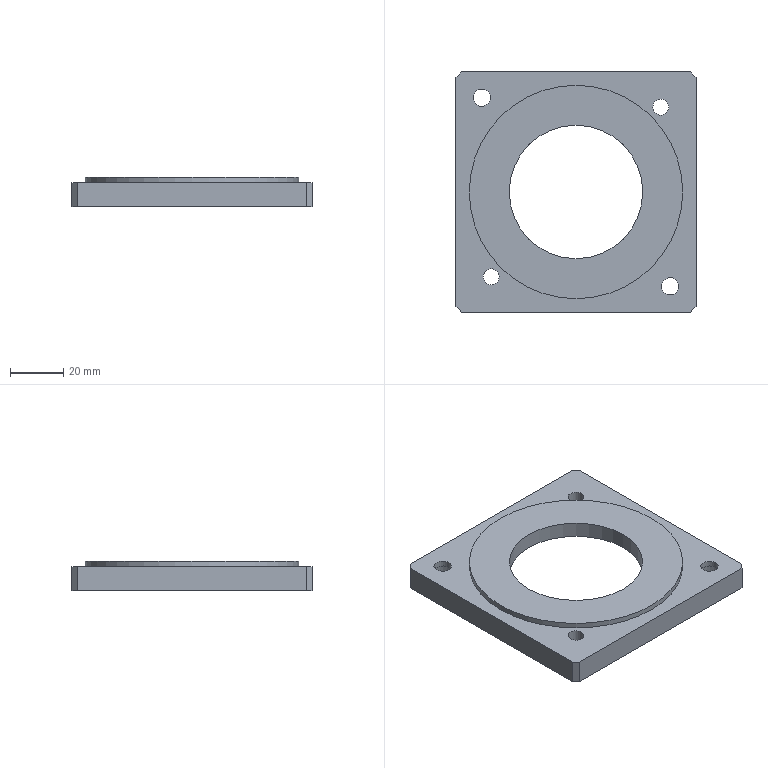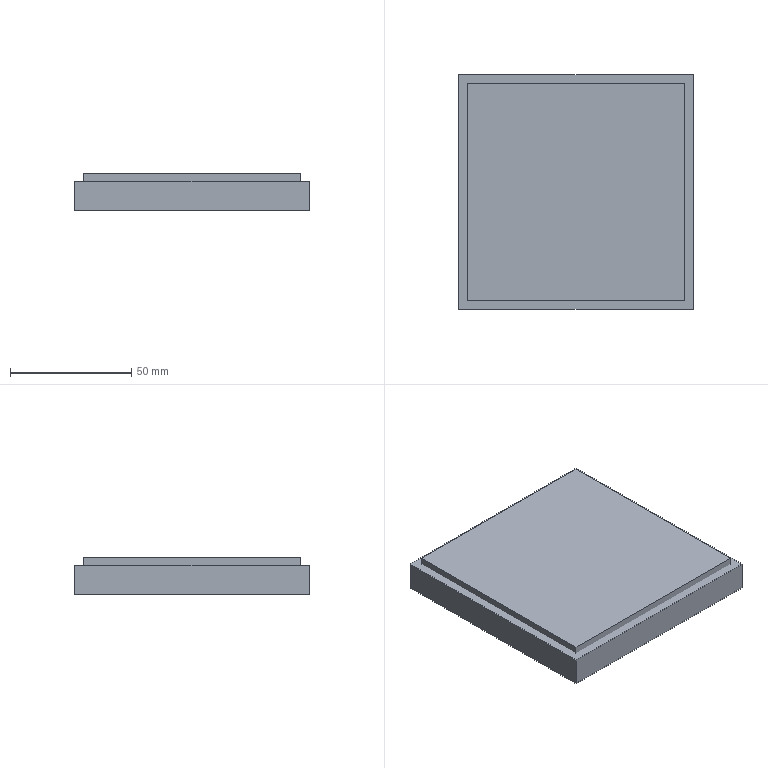CAM job | NX | 3-axis milling, drilling | part box 90 x 90 x 11 mm | stock box 97 x 97 x 15 mm
Tools:
number,name,description,diameter,corner_radius,flute_length,length,flutes
10,D10,Milling Tool-5 Parameters,10.0,0.0,50.0,75.0,2
7,D6A45,Milling Tool-5 Parameters,6.0,0.0,3.0,3.0,2
3,6.5ZT,Drilling Tool,6.5,0.0,35.0,50.0,2
4,5.0ZT,Drilling Tool,5.0,0.0,35.0,50.0,2
6,D6,Milling Tool-5 Parameters,6.0,0.0,50.0,75.0,2
15,D50,Milling Tool-5 Parameters,50.0,0.0,50.0,75.0,2
Operations:
program,operation,operation_type,tool,method,geometry_group,spindle_rpm,surface_speed,feed_per_tooth,feed_cut,feed_plunge,cut_length_mm,path_length_mm,cut_time_min,machine_time_min
1,FLOOR_WALL,VolumeBased25DMillingOperation,D50,METHOD,A,6500.0,1286.0,0.0962,1250.0,100.0,529.997,583.997,0.424,0.4294
1,ADAPTIVE_MILLING,CavityMilling,D10,METHOD,A,9500.0,298.0,0.1579,3000.0,1000.0,9181.397,9428.795,3.599,3.624
1,DRILLING,Operation,D6A45,METHOD,A,3000.0,56.0,0.0333,200.0,0.0,16.0,307.005,0.08,0.1091
1,DRILLING_COPY,Operation,6.5ZT,METHOD,A,1500.0,42.0,0.0667,200.0,0.0,27.906,222.856,0.1395,0.159
1,DRILLING_COPY_COPY,Operation,5.0ZT,METHOD,A,1500.0,42.0,0.0667,200.0,0.0,30.004,217.059,0.15,0.1687
1,ZLEVEL_PROFILE,ZLevelMilling,D10,METHOD,A,9000.0,282.0,0.0556,1000.0,100.0,535.495,742.123,0.5355,0.5562
1,FLOOR_WALL_1,VolumeBased25DMillingOperation,D10,METHOD,A,9500.0,298.0,0.0658,1250.0,100.0,1161.072,1475.491,0.9289,0.9603
1,ZLEVEL_PROFILE_COPY_1_COPY_COPY_COPY_COPY_2_COPY,ZLevelMilling,D6A45,METHOD,A,7000.0,131.0,0.0714,1000.0,1000.0,415.104,558.433,0.4151,0.4294
1,ZLEVEL_PROFILE_COPY_1_COPY_COPY_COPY_COPY_2_COPY_COPY,ZLevelMilling,D6A45,METHOD,A,7000.0,131.0,0.0714,1000.0,1000.0,426.989,1027.141,0.427,0.487
1,刀补10,VolumeBased25DMillingOperation,D10,METHOD,A,9500.0,298.0,0.0658,1250.0,100.0,290.077,351.077,0.2321,0.2382
2,FLOOR_WALL_COPY,VolumeBased25DMillingOperation,D50,METHOD,B,6500.0,1286.0,0.0962,1250.0,100.0,2007.988,2697.726,1.606,1.675
2,HOLE_MILLING_COPY,CylinderMilling,D10,METHOD,B,9500.0,298.0,0.1579,3000.0,100.0,2265.933,2330.333,0.7553,0.7618
2,FLOOR_WALL_1_COPY,VolumeBased25DMillingOperation,D10,METHOD,B,9500.0,298.0,0.0658,1250.0,100.0,381.525,448.525,0.3052,0.3119
2,HOLE_MILLING,CylinderMilling,D6,METHOD,B,9500.0,179.0,0.0737,1400.0,100.0,506.029,738.629,0.3614,0.3847
2,ZLEVEL_PROFILE_COPY_1_COPY_COPY_COPY_COPY_2_COPY_COPY_1,ZLevelMilling,D6A45,METHOD,B,7000.0,131.0,0.0714,1000.0,1000.0,678.457,1464.339,0.6785,0.757
2,ZLEVEL_PROFILE_COPY_1_COPY_COPY_COPY_COPY_2_COPY_COPY_1_COPY,ZLevelMilling,D6A45,METHOD,B,7000.0,131.0,0.0714,1000.0,1000.0,154.448,226.448,0.1544,0.1616
2,刀补10_COPY,VolumeBased25DMillingOperation,D10,METHOD,B,9500.0,298.0,0.0658,1250.0,100.0,195.586,262.586,0.1565,0.1632